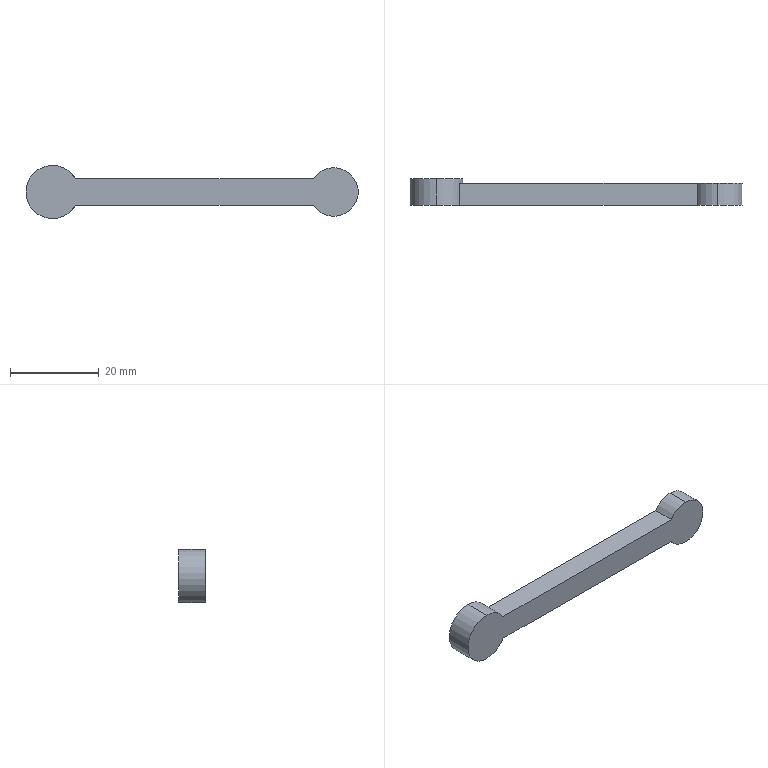Part | STEP file | 111_Default | 1 solid | 10 faces | box 75 x 6 x 12 mm | volume 2730 mm3 | cylinder 5 | plane 5 | commonest cylinder face diameters 11 x3 12 x2
STEP:
#1=CARTESIAN_POINT('',(0.,0.,0.));
#2=DIRECTION('',(0.,0.,1.));
#3=DIRECTION('',(1.,0.,0.));
#4=AXIS2_PLACEMENT_3D('',#1,#2,#3);
#5=CARTESIAN_POINT('',(31.75,0.,5.5));
#6=VERTEX_POINT('',#5);
#7=CARTESIAN_POINT('',(31.75,0.,-5.5));
#8=VERTEX_POINT('',#7);
#9=CARTESIAN_POINT('',(31.75,0.,0.));
#10=DIRECTION('',(0.,1.,0.));
#11=DIRECTION('',(0.,0.,1.));
#12=AXIS2_PLACEMENT_3D('',#9,#10,#11);
#13=CIRCLE('',#12,5.5);
#14=CARTESIAN_POINT('',(31.75,-5.,0.));
#15=DIRECTION('',(0.,1.,0.));
#16=DIRECTION('',(0.,0.,1.));
#17=AXIS2_PLACEMENT_3D('',#14,#15,#16);
#18=CYLINDRICAL_SURFACE('',#17,5.5);
#19=CARTESIAN_POINT('',(0.,5.));
#20=DIRECTION('',(1.,0.));
#21=VECTOR('',#20,1.);
#22=LINE('',#19,#21);
#23=(GEOMETRIC_REPRESENTATION_CONTEXT(2)PARAMETRIC_REPRESENTATION_CONTEXT()REPRESENTATION_CONTEXT('',''));
#24=DEFINITIONAL_REPRESENTATION('',(#22),#23);
#25=PCURVE('',#18,#24);
#26=CARTESIAN_POINT('',(31.75,0.,0.));
#27=DIRECTION('',(0.,1.,0.));
#28=DIRECTION('',(0.,0.,1.));
#29=AXIS2_PLACEMENT_3D('',#26,#27,#28);
#30=PLANE('',#29);
#31=CARTESIAN_POINT('',(0.,0.));
#32=DIRECTION('',(1.,0.));
#33=AXIS2_PLACEMENT_2D('',#31,#32);
#34=CIRCLE('',#33,5.5);
#35=(GEOMETRIC_REPRESENTATION_CONTEXT(2)PARAMETRIC_REPRESENTATION_CONTEXT()REPRESENTATION_CONTEXT('',''));
#36=DEFINITIONAL_REPRESENTATION('',(#34),#35);
#37=PCURVE('',#30,#36);
#38=SURFACE_CURVE('',#13,(#25,#37),.PCURVE_S1.);
#39=EDGE_CURVE('',#6,#8,#38,.T.);
#40=ORIENTED_EDGE('',*,*,#39,.T.);
#41=CARTESIAN_POINT('',(31.75,5.,-5.5));
#42=VERTEX_POINT('',#41);
#43=CARTESIAN_POINT('',(31.75,-5.,-5.5));
#44=DIRECTION('',(0.,1.,0.));
#45=VECTOR('',#44,1.);
#46=LINE('',#43,#45);
#47=CARTESIAN_POINT('',(3.142,0.));
#48=DIRECTION('',(0.,1.));
#49=VECTOR('',#48,1.);
#50=LINE('',#47,#49);
#51=(GEOMETRIC_REPRESENTATION_CONTEXT(2)PARAMETRIC_REPRESENTATION_CONTEXT()REPRESENTATION_CONTEXT('',''));
#52=DEFINITIONAL_REPRESENTATION('',(#50),#51);
#53=PCURVE('',#18,#52);
#54=CARTESIAN_POINT('',(31.75,-5.,0.));
#55=DIRECTION('',(0.,1.,0.));
#56=DIRECTION('',(0.,0.,1.));
#57=AXIS2_PLACEMENT_3D('',#54,#55,#56);
#58=CYLINDRICAL_SURFACE('',#57,5.5);
#59=CARTESIAN_POINT('',(3.142,0.));
#60=DIRECTION('',(0.,1.));
#61=VECTOR('',#60,1.);
#62=LINE('',#59,#61);
#63=(GEOMETRIC_REPRESENTATION_CONTEXT(2)PARAMETRIC_REPRESENTATION_CONTEXT()REPRESENTATION_CONTEXT('',''));
#64=DEFINITIONAL_REPRESENTATION('',(#62),#63);
#65=PCURVE('',#58,#64);
#66=SURFACE_CURVE('',#46,(#53,#65),.PCURVE_S1.);
#67=EDGE_CURVE('',#8,#42,#66,.T.);
#68=ORIENTED_EDGE('',*,*,#67,.T.);
#69=CARTESIAN_POINT('',(31.75,5.,5.5));
#70=VERTEX_POINT('',#69);
#71=CARTESIAN_POINT('',(31.75,5.,0.));
#72=DIRECTION('',(0.,1.,0.));
#73=DIRECTION('',(0.,0.,1.));
#74=AXIS2_PLACEMENT_3D('',#71,#72,#73);
#75=CIRCLE('',#74,5.5);
#76=CARTESIAN_POINT('',(0.,10.));
#77=DIRECTION('',(1.,0.));
#78=VECTOR('',#77,1.);
#79=LINE('',#76,#78);
#80=(GEOMETRIC_REPRESENTATION_CONTEXT(2)PARAMETRIC_REPRESENTATION_CONTEXT()REPRESENTATION_CONTEXT('',''));
#81=DEFINITIONAL_REPRESENTATION('',(#79),#80);
#82=PCURVE('',#18,#81);
#83=CARTESIAN_POINT('',(31.75,5.,0.));
#84=DIRECTION('',(0.,1.,0.));
#85=DIRECTION('',(0.,0.,1.));
#86=AXIS2_PLACEMENT_3D('',#83,#84,#85);
#87=PLANE('',#86);
#88=CARTESIAN_POINT('',(0.,0.));
#89=DIRECTION('',(1.,0.));
#90=AXIS2_PLACEMENT_2D('',#88,#89);
#91=CIRCLE('',#90,5.5);
#92=(GEOMETRIC_REPRESENTATION_CONTEXT(2)PARAMETRIC_REPRESENTATION_CONTEXT()REPRESENTATION_CONTEXT('',''));
#93=DEFINITIONAL_REPRESENTATION('',(#91),#92);
#94=PCURVE('',#87,#93);
#95=SURFACE_CURVE('',#75,(#82,#94),.PCURVE_S1.);
#96=EDGE_CURVE('',#70,#42,#95,.T.);
#97=ORIENTED_EDGE('',*,*,#96,.F.);
#98=CARTESIAN_POINT('',(31.75,-5.,5.5));
#99=DIRECTION('',(0.,1.,0.));
#100=VECTOR('',#99,1.);
#101=LINE('',#98,#100);
#102=CARTESIAN_POINT('',(0.,0.));
#103=DIRECTION('',(0.,1.));
#104=VECTOR('',#103,1.);
#105=LINE('',#102,#104);
#106=(GEOMETRIC_REPRESENTATION_CONTEXT(2)PARAMETRIC_REPRESENTATION_CONTEXT()REPRESENTATION_CONTEXT('',''));
#107=DEFINITIONAL_REPRESENTATION('',(#105),#106);
#108=PCURVE('',#18,#107);
#109=CARTESIAN_POINT('',(31.75,-5.,0.));
#110=DIRECTION('',(0.,1.,0.));
#111=DIRECTION('',(0.,0.,1.));
#112=AXIS2_PLACEMENT_3D('',#109,#110,#111);
#113=CYLINDRICAL_SURFACE('',#112,5.5);
#114=CARTESIAN_POINT('',(6.283,0.));
#115=DIRECTION('',(0.,1.));
#116=VECTOR('',#115,1.);
#117=LINE('',#114,#116);
#118=(GEOMETRIC_REPRESENTATION_CONTEXT(2)PARAMETRIC_REPRESENTATION_CONTEXT()REPRESENTATION_CONTEXT('',''));
#119=DEFINITIONAL_REPRESENTATION('',(#117),#118);
#120=PCURVE('',#113,#119);
#121=SURFACE_CURVE('',#101,(#108,#120),.PCURVE_S1.);
#122=EDGE_CURVE('',#6,#70,#121,.T.);
#123=ORIENTED_EDGE('',*,*,#122,.F.);
#124=EDGE_LOOP('',(#40,#68,#97,#123));
#125=FACE_BOUND('',#124,.T.);
#126=ADVANCED_FACE('',(#125),#18,.T.);
#127=CARTESIAN_POINT('',(27.14,0.,3.));
#128=VERTEX_POINT('',#127);
#129=CARTESIAN_POINT('',(31.75,0.,0.));
#130=DIRECTION('',(0.,1.,0.));
#131=DIRECTION('',(0.,0.,1.));
#132=AXIS2_PLACEMENT_3D('',#129,#130,#131);
#133=CIRCLE('',#132,5.5);
#134=CARTESIAN_POINT('',(0.,5.));
#135=DIRECTION('',(1.,0.));
#136=VECTOR('',#135,1.);
#137=LINE('',#134,#136);
#138=(GEOMETRIC_REPRESENTATION_CONTEXT(2)PARAMETRIC_REPRESENTATION_CONTEXT()REPRESENTATION_CONTEXT('',''));
#139=DEFINITIONAL_REPRESENTATION('',(#137),#138);
#140=PCURVE('',#113,#139);
#141=CARTESIAN_POINT('',(0.,0.));
#142=DIRECTION('',(1.,0.));
#143=AXIS2_PLACEMENT_2D('',#141,#142);
#144=CIRCLE('',#143,5.5);
#145=(GEOMETRIC_REPRESENTATION_CONTEXT(2)PARAMETRIC_REPRESENTATION_CONTEXT()REPRESENTATION_CONTEXT('',''));
#146=DEFINITIONAL_REPRESENTATION('',(#144),#145);
#147=PCURVE('',#30,#146);
#148=SURFACE_CURVE('',#133,(#140,#147),.PCURVE_S1.);
#149=EDGE_CURVE('',#128,#6,#148,.T.);
#150=ORIENTED_EDGE('',*,*,#149,.T.);
#151=ORIENTED_EDGE('',*,*,#122,.T.);
#152=CARTESIAN_POINT('',(27.14,5.,3.));
#153=VERTEX_POINT('',#152);
#154=CARTESIAN_POINT('',(31.75,5.,0.));
#155=DIRECTION('',(0.,1.,0.));
#156=DIRECTION('',(0.,0.,1.));
#157=AXIS2_PLACEMENT_3D('',#154,#155,#156);
#158=CIRCLE('',#157,5.5);
#159=CARTESIAN_POINT('',(0.,10.));
#160=DIRECTION('',(1.,0.));
#161=VECTOR('',#160,1.);
#162=LINE('',#159,#161);
#163=(GEOMETRIC_REPRESENTATION_CONTEXT(2)PARAMETRIC_REPRESENTATION_CONTEXT()REPRESENTATION_CONTEXT('',''));
#164=DEFINITIONAL_REPRESENTATION('',(#162),#163);
#165=PCURVE('',#113,#164);
#166=CARTESIAN_POINT('',(0.,0.));
#167=DIRECTION('',(1.,0.));
#168=AXIS2_PLACEMENT_2D('',#166,#167);
#169=CIRCLE('',#168,5.5);
#170=(GEOMETRIC_REPRESENTATION_CONTEXT(2)PARAMETRIC_REPRESENTATION_CONTEXT()REPRESENTATION_CONTEXT('',''));
#171=DEFINITIONAL_REPRESENTATION('',(#169),#170);
#172=PCURVE('',#87,#171);
#173=SURFACE_CURVE('',#158,(#165,#172),.PCURVE_S1.);
#174=EDGE_CURVE('',#153,#70,#173,.T.);
#175=ORIENTED_EDGE('',*,*,#174,.F.);
#176=CARTESIAN_POINT('',(27.14,-5.,3.));
#177=DIRECTION('',(0.,1.,0.));
#178=VECTOR('',#177,1.);
#179=LINE('',#176,#178);
#180=CARTESIAN_POINT('',(5.289,0.));
#181=DIRECTION('',(0.,1.));
#182=VECTOR('',#181,1.);
#183=LINE('',#180,#182);
#184=(GEOMETRIC_REPRESENTATION_CONTEXT(2)PARAMETRIC_REPRESENTATION_CONTEXT()REPRESENTATION_CONTEXT('',''));
#185=DEFINITIONAL_REPRESENTATION('',(#183),#184);
#186=PCURVE('',#113,#185);
#187=CARTESIAN_POINT('',(-26.554,-5.,3.));
#188=DIRECTION('',(0.,0.,1.));
#189=DIRECTION('',(1.,0.,0.));
#190=AXIS2_PLACEMENT_3D('',#187,#188,#189);
#191=PLANE('',#190);
#192=CARTESIAN_POINT('',(53.694,0.));
#193=DIRECTION('',(0.,1.));
#194=VECTOR('',#193,1.);
#195=LINE('',#192,#194);
#196=(GEOMETRIC_REPRESENTATION_CONTEXT(2)PARAMETRIC_REPRESENTATION_CONTEXT()REPRESENTATION_CONTEXT('',''));
#197=DEFINITIONAL_REPRESENTATION('',(#195),#196);
#198=PCURVE('',#191,#197);
#199=SURFACE_CURVE('',#179,(#186,#198),.PCURVE_S1.);
#200=EDGE_CURVE('',#128,#153,#199,.T.);
#201=ORIENTED_EDGE('',*,*,#200,.F.);
#202=EDGE_LOOP('',(#150,#151,#175,#201));
#203=FACE_BOUND('',#202,.T.);
#204=ADVANCED_FACE('',(#203),#113,.T.);
#205=CARTESIAN_POINT('',(-31.75,6.,6.));
#206=VERTEX_POINT('',#205);
#207=CARTESIAN_POINT('',(-31.75,6.,-6.));
#208=VERTEX_POINT('',#207);
#209=CARTESIAN_POINT('',(-31.75,6.,0.));
#210=DIRECTION('',(0.,1.,0.));
#211=DIRECTION('',(0.,0.,1.));
#212=AXIS2_PLACEMENT_3D('',#209,#210,#211);
#213=CIRCLE('',#212,6.);
#214=CARTESIAN_POINT('',(-31.75,5.,0.));
#215=DIRECTION('',(0.,-1.,0.));
#216=DIRECTION('',(0.,0.,-1.));
#217=AXIS2_PLACEMENT_3D('',#214,#215,#216);
#218=CYLINDRICAL_SURFACE('',#217,6.);
#219=CARTESIAN_POINT('',(3.142,-1.));
#220=DIRECTION('',(-1.,0.));
#221=VECTOR('',#220,1.);
#222=LINE('',#219,#221);
#223=(GEOMETRIC_REPRESENTATION_CONTEXT(2)PARAMETRIC_REPRESENTATION_CONTEXT()REPRESENTATION_CONTEXT('',''));
#224=DEFINITIONAL_REPRESENTATION('',(#222),#223);
#225=PCURVE('',#218,#224);
#226=CARTESIAN_POINT('',(-31.75,6.,0.));
#227=DIRECTION('',(0.,1.,0.));
#228=DIRECTION('',(0.,0.,1.));
#229=AXIS2_PLACEMENT_3D('',#226,#227,#228);
#230=PLANE('',#229);
#231=CARTESIAN_POINT('',(0.,0.));
#232=DIRECTION('',(1.,0.));
#233=AXIS2_PLACEMENT_2D('',#231,#232);
#234=CIRCLE('',#233,6.);
#235=(GEOMETRIC_REPRESENTATION_CONTEXT(2)PARAMETRIC_REPRESENTATION_CONTEXT()REPRESENTATION_CONTEXT('',''));
#236=DEFINITIONAL_REPRESENTATION('',(#234),#235);
#237=PCURVE('',#230,#236);
#238=SURFACE_CURVE('',#213,(#225,#237),.PCURVE_S1.);
#239=EDGE_CURVE('',#206,#208,#238,.T.);
#240=ORIENTED_EDGE('',*,*,#239,.F.);
#241=CARTESIAN_POINT('',(-31.75,0.,6.));
#242=VERTEX_POINT('',#241);
#243=CARTESIAN_POINT('',(-31.75,5.,6.));
#244=DIRECTION('',(0.,-1.,0.));
#245=VECTOR('',#244,1.);
#246=LINE('',#243,#245);
#247=CARTESIAN_POINT('',(3.142,0.));
#248=DIRECTION('',(0.,1.));
#249=VECTOR('',#248,1.);
#250=LINE('',#247,#249);
#251=(GEOMETRIC_REPRESENTATION_CONTEXT(2)PARAMETRIC_REPRESENTATION_CONTEXT()REPRESENTATION_CONTEXT('',''));
#252=DEFINITIONAL_REPRESENTATION('',(#250),#251);
#253=PCURVE('',#218,#252);
#254=CARTESIAN_POINT('',(-31.75,5.,0.));
#255=DIRECTION('',(0.,-1.,0.));
#256=DIRECTION('',(0.,0.,-1.));
#257=AXIS2_PLACEMENT_3D('',#254,#255,#256);
#258=CYLINDRICAL_SURFACE('',#257,6.);
#259=CARTESIAN_POINT('',(3.142,0.));
#260=DIRECTION('',(0.,1.));
#261=VECTOR('',#260,1.);
#262=LINE('',#259,#261);
#263=(GEOMETRIC_REPRESENTATION_CONTEXT(2)PARAMETRIC_REPRESENTATION_CONTEXT()REPRESENTATION_CONTEXT('',''));
#264=DEFINITIONAL_REPRESENTATION('',(#262),#263);
#265=PCURVE('',#258,#264);
#266=SURFACE_CURVE('',#246,(#253,#265),.PCURVE_S1.);
#267=EDGE_CURVE('',#206,#242,#266,.T.);
#268=ORIENTED_EDGE('',*,*,#267,.T.);
#269=CARTESIAN_POINT('',(-26.554,0.,3.));
#270=VERTEX_POINT('',#269);
#271=CARTESIAN_POINT('',(-31.75,0.,0.));
#272=DIRECTION('',(0.,1.,0.));
#273=DIRECTION('',(0.,0.,1.));
#274=AXIS2_PLACEMENT_3D('',#271,#272,#273);
#275=CIRCLE('',#274,6.);
#276=CARTESIAN_POINT('',(3.142,5.));
#277=DIRECTION('',(-1.,0.));
#278=VECTOR('',#277,1.);
#279=LINE('',#276,#278);
#280=(GEOMETRIC_REPRESENTATION_CONTEXT(2)PARAMETRIC_REPRESENTATION_CONTEXT()REPRESENTATION_CONTEXT('',''));
#281=DEFINITIONAL_REPRESENTATION('',(#279),#280);
#282=PCURVE('',#218,#281);
#283=CARTESIAN_POINT('',(0.,-63.5));
#284=DIRECTION('',(1.,0.));
#285=AXIS2_PLACEMENT_2D('',#283,#284);
#286=CIRCLE('',#285,6.);
#287=(GEOMETRIC_REPRESENTATION_CONTEXT(2)PARAMETRIC_REPRESENTATION_CONTEXT()REPRESENTATION_CONTEXT('',''));
#288=DEFINITIONAL_REPRESENTATION('',(#286),#287);
#289=PCURVE('',#30,#288);
#290=SURFACE_CURVE('',#275,(#282,#289),.PCURVE_S1.);
#291=EDGE_CURVE('',#242,#270,#290,.T.);
#292=ORIENTED_EDGE('',*,*,#291,.T.);
#293=CARTESIAN_POINT('',(-26.554,5.,3.));
#294=VERTEX_POINT('',#293);
#295=CARTESIAN_POINT('',(-26.554,-5.,3.));
#296=DIRECTION('',(0.,1.,0.));
#297=VECTOR('',#296,1.);
#298=LINE('',#295,#297);
#299=CARTESIAN_POINT('',(2.094,10.));
#300=DIRECTION('',(0.,-1.));
#301=VECTOR('',#300,1.);
#302=LINE('',#299,#301);
#303=(GEOMETRIC_REPRESENTATION_CONTEXT(2)PARAMETRIC_REPRESENTATION_CONTEXT()REPRESENTATION_CONTEXT('',''));
#304=DEFINITIONAL_REPRESENTATION('',(#302),#303);
#305=PCURVE('',#218,#304);
#306=CARTESIAN_POINT('',(0.,0.));
#307=DIRECTION('',(0.,1.));
#308=VECTOR('',#307,1.);
#309=LINE('',#306,#308);
#310=(GEOMETRIC_REPRESENTATION_CONTEXT(2)PARAMETRIC_REPRESENTATION_CONTEXT()REPRESENTATION_CONTEXT('',''));
#311=DEFINITIONAL_REPRESENTATION('',(#309),#310);
#312=PCURVE('',#191,#311);
#313=SURFACE_CURVE('',#298,(#305,#312),.PCURVE_S1.);
#314=EDGE_CURVE('',#270,#294,#313,.T.);
#315=ORIENTED_EDGE('',*,*,#314,.T.);
#316=CARTESIAN_POINT('',(-26.554,5.,-3.));
#317=VERTEX_POINT('',#316);
#318=CARTESIAN_POINT('',(-31.75,5.,0.));
#319=DIRECTION('',(0.,1.,0.));
#320=DIRECTION('',(0.,0.,1.));
#321=AXIS2_PLACEMENT_3D('',#318,#319,#320);
#322=CIRCLE('',#321,6.);
#323=CARTESIAN_POINT('',(3.142,0.));
#324=DIRECTION('',(-1.,0.));
#325=VECTOR('',#324,1.);
#326=LINE('',#323,#325);
#327=(GEOMETRIC_REPRESENTATION_CONTEXT(2)PARAMETRIC_REPRESENTATION_CONTEXT()REPRESENTATION_CONTEXT('',''));
#328=DEFINITIONAL_REPRESENTATION('',(#326),#327);
#329=PCURVE('',#218,#328);
#330=CARTESIAN_POINT('',(0.,-63.5));
#331=DIRECTION('',(1.,0.));
#332=AXIS2_PLACEMENT_2D('',#330,#331);
#333=CIRCLE('',#332,6.);
#334=(GEOMETRIC_REPRESENTATION_CONTEXT(2)PARAMETRIC_REPRESENTATION_CONTEXT()REPRESENTATION_CONTEXT('',''));
#335=DEFINITIONAL_REPRESENTATION('',(#333),#334);
#336=PCURVE('',#87,#335);
#337=SURFACE_CURVE('',#322,(#329,#336),.PCURVE_S1.);
#338=EDGE_CURVE('',#294,#317,#337,.T.);
#339=ORIENTED_EDGE('',*,*,#338,.T.);
#340=CARTESIAN_POINT('',(-26.554,0.,-3.));
#341=VERTEX_POINT('',#340);
#342=CARTESIAN_POINT('',(-26.554,-5.,-3.));
#343=DIRECTION('',(0.,1.,0.));
#344=VECTOR('',#343,1.);
#345=LINE('',#342,#344);
#346=CARTESIAN_POINT('',(1.047,10.));
#347=DIRECTION('',(0.,-1.));
#348=VECTOR('',#347,1.);
#349=LINE('',#346,#348);
#350=(GEOMETRIC_REPRESENTATION_CONTEXT(2)PARAMETRIC_REPRESENTATION_CONTEXT()REPRESENTATION_CONTEXT('',''));
#351=DEFINITIONAL_REPRESENTATION('',(#349),#350);
#352=PCURVE('',#218,#351);
#353=CARTESIAN_POINT('',(-26.554,-5.,-3.));
#354=DIRECTION('',(0.,0.,-1.));
#355=DIRECTION('',(-1.,0.,0.));
#356=AXIS2_PLACEMENT_3D('',#353,#354,#355);
#357=PLANE('',#356);
#358=CARTESIAN_POINT('',(0.,0.));
#359=DIRECTION('',(0.,1.));
#360=VECTOR('',#359,1.);
#361=LINE('',#358,#360);
#362=(GEOMETRIC_REPRESENTATION_CONTEXT(2)PARAMETRIC_REPRESENTATION_CONTEXT()REPRESENTATION_CONTEXT('',''));
#363=DEFINITIONAL_REPRESENTATION('',(#361),#362);
#364=PCURVE('',#357,#363);
#365=SURFACE_CURVE('',#345,(#352,#364),.PCURVE_S1.);
#366=EDGE_CURVE('',#341,#317,#365,.T.);
#367=ORIENTED_EDGE('',*,*,#366,.F.);
#368=CARTESIAN_POINT('',(-31.75,0.,-6.));
#369=VERTEX_POINT('',#368);
#370=CARTESIAN_POINT('',(-31.75,0.,0.));
#371=DIRECTION('',(0.,1.,0.));
#372=DIRECTION('',(0.,0.,1.));
#373=AXIS2_PLACEMENT_3D('',#370,#371,#372);
#374=CIRCLE('',#373,6.);
#375=CARTESIAN_POINT('',(3.142,5.));
#376=DIRECTION('',(-1.,0.));
#377=VECTOR('',#376,1.);
#378=LINE('',#375,#377);
#379=(GEOMETRIC_REPRESENTATION_CONTEXT(2)PARAMETRIC_REPRESENTATION_CONTEXT()REPRESENTATION_CONTEXT('',''));
#380=DEFINITIONAL_REPRESENTATION('',(#378),#379);
#381=PCURVE('',#218,#380);
#382=CARTESIAN_POINT('',(0.,-63.5));
#383=DIRECTION('',(1.,0.));
#384=AXIS2_PLACEMENT_2D('',#382,#383);
#385=CIRCLE('',#384,6.);
#386=(GEOMETRIC_REPRESENTATION_CONTEXT(2)PARAMETRIC_REPRESENTATION_CONTEXT()REPRESENTATION_CONTEXT('',''));
#387=DEFINITIONAL_REPRESENTATION('',(#385),#386);
#388=PCURVE('',#30,#387);
#389=SURFACE_CURVE('',#374,(#381,#388),.PCURVE_S1.);
#390=EDGE_CURVE('',#341,#369,#389,.T.);
#391=ORIENTED_EDGE('',*,*,#390,.T.);
#392=CARTESIAN_POINT('',(-31.75,5.,-6.));
#393=DIRECTION('',(0.,-1.,0.));
#394=VECTOR('',#393,1.);
#395=LINE('',#392,#394);
#396=CARTESIAN_POINT('',(0.,0.));
#397=DIRECTION('',(0.,1.));
#398=VECTOR('',#397,1.);
#399=LINE('',#396,#398);
#400=(GEOMETRIC_REPRESENTATION_CONTEXT(2)PARAMETRIC_REPRESENTATION_CONTEXT()REPRESENTATION_CONTEXT('',''));
#401=DEFINITIONAL_REPRESENTATION('',(#399),#400);
#402=PCURVE('',#218,#401);
#403=CARTESIAN_POINT('',(6.283,0.));
#404=DIRECTION('',(0.,1.));
#405=VECTOR('',#404,1.);
#406=LINE('',#403,#405);
#407=(GEOMETRIC_REPRESENTATION_CONTEXT(2)PARAMETRIC_REPRESENTATION_CONTEXT()REPRESENTATION_CONTEXT('',''));
#408=DEFINITIONAL_REPRESENTATION('',(#406),#407);
#409=PCURVE('',#258,#408);
#410=SURFACE_CURVE('',#395,(#402,#409),.PCURVE_S1.);
#411=EDGE_CURVE('',#208,#369,#410,.T.);
#412=ORIENTED_EDGE('',*,*,#411,.F.);
#413=EDGE_LOOP('',(#240,#268,#292,#315,#339,#367,#391,#412));
#414=FACE_BOUND('',#413,.T.);
#415=ADVANCED_FACE('',(#414),#218,.T.);
#416=ORIENTED_EDGE('',*,*,#338,.F.);
#417=CARTESIAN_POINT('',(-26.554,5.,3.));
#418=DIRECTION('',(1.,0.,0.));
#419=VECTOR('',#418,1.);
#420=LINE('',#417,#419);
#421=CARTESIAN_POINT('',(3.,-58.304));
#422=DIRECTION('',(0.,1.));
#423=VECTOR('',#422,1.);
#424=LINE('',#421,#423);
#425=(GEOMETRIC_REPRESENTATION_CONTEXT(2)PARAMETRIC_REPRESENTATION_CONTEXT()REPRESENTATION_CONTEXT('',''));
#426=DEFINITIONAL_REPRESENTATION('',(#424),#425);
#427=PCURVE('',#87,#426);
#428=CARTESIAN_POINT('',(0.,10.));
#429=DIRECTION('',(1.,0.));
#430=VECTOR('',#429,1.);
#431=LINE('',#428,#430);
#432=(GEOMETRIC_REPRESENTATION_CONTEXT(2)PARAMETRIC_REPRESENTATION_CONTEXT()REPRESENTATION_CONTEXT('',''));
#433=DEFINITIONAL_REPRESENTATION('',(#431),#432);
#434=PCURVE('',#191,#433);
#435=SURFACE_CURVE('',#420,(#427,#434),.PCURVE_S1.);
#436=EDGE_CURVE('',#294,#153,#435,.T.);
#437=ORIENTED_EDGE('',*,*,#436,.T.);
#438=ORIENTED_EDGE('',*,*,#174,.T.);
#439=ORIENTED_EDGE('',*,*,#96,.T.);
#440=CARTESIAN_POINT('',(27.14,5.,-3.));
#441=VERTEX_POINT('',#440);
#442=CARTESIAN_POINT('',(31.75,5.,0.));
#443=DIRECTION('',(0.,1.,0.));
#444=DIRECTION('',(0.,0.,1.));
#445=AXIS2_PLACEMENT_3D('',#442,#443,#444);
#446=CIRCLE('',#445,5.5);
#447=CARTESIAN_POINT('',(0.,0.));
#448=DIRECTION('',(1.,0.));
#449=AXIS2_PLACEMENT_2D('',#447,#448);
#450=CIRCLE('',#449,5.5);
#451=(GEOMETRIC_REPRESENTATION_CONTEXT(2)PARAMETRIC_REPRESENTATION_CONTEXT()REPRESENTATION_CONTEXT('',''));
#452=DEFINITIONAL_REPRESENTATION('',(#450),#451);
#453=PCURVE('',#87,#452);
#454=CARTESIAN_POINT('',(0.,10.));
#455=DIRECTION('',(1.,0.));
#456=VECTOR('',#455,1.);
#457=LINE('',#454,#456);
#458=(GEOMETRIC_REPRESENTATION_CONTEXT(2)PARAMETRIC_REPRESENTATION_CONTEXT()REPRESENTATION_CONTEXT('',''));
#459=DEFINITIONAL_REPRESENTATION('',(#457),#458);
#460=PCURVE('',#58,#459);
#461=SURFACE_CURVE('',#446,(#453,#460),.PCURVE_S1.);
#462=EDGE_CURVE('',#42,#441,#461,.T.);
#463=ORIENTED_EDGE('',*,*,#462,.T.);
#464=CARTESIAN_POINT('',(-26.554,5.,-3.));
#465=DIRECTION('',(-1.,0.,0.));
#466=VECTOR('',#465,1.);
#467=LINE('',#464,#466);
#468=CARTESIAN_POINT('',(-3.,-58.304));
#469=DIRECTION('',(0.,-1.));
#470=VECTOR('',#469,1.);
#471=LINE('',#468,#470);
#472=(GEOMETRIC_REPRESENTATION_CONTEXT(2)PARAMETRIC_REPRESENTATION_CONTEXT()REPRESENTATION_CONTEXT('',''));
#473=DEFINITIONAL_REPRESENTATION('',(#471),#472);
#474=PCURVE('',#87,#473);
#475=CARTESIAN_POINT('',(0.,10.));
#476=DIRECTION('',(1.,0.));
#477=VECTOR('',#476,1.);
#478=LINE('',#475,#477);
#479=(GEOMETRIC_REPRESENTATION_CONTEXT(2)PARAMETRIC_REPRESENTATION_CONTEXT()REPRESENTATION_CONTEXT('',''));
#480=DEFINITIONAL_REPRESENTATION('',(#478),#479);
#481=PCURVE('',#357,#480);
#482=SURFACE_CURVE('',#467,(#474,#481),.PCURVE_S1.);
#483=EDGE_CURVE('',#441,#317,#482,.T.);
#484=ORIENTED_EDGE('',*,*,#483,.T.);
#485=EDGE_LOOP('',(#416,#437,#438,#439,#463,#484));
#486=FACE_BOUND('',#485,.T.);
#487=ADVANCED_FACE('',(#486),#87,.T.);
#488=ORIENTED_EDGE('',*,*,#390,.F.);
#489=CARTESIAN_POINT('',(27.14,0.,-3.));
#490=VERTEX_POINT('',#489);
#491=CARTESIAN_POINT('',(31.75,0.,-3.));
#492=DIRECTION('',(-1.,0.,0.));
#493=VECTOR('',#492,1.);
#494=LINE('',#491,#493);
#495=CARTESIAN_POINT('',(-3.,0.));
#496=DIRECTION('',(0.,-1.));
#497=VECTOR('',#496,1.);
#498=LINE('',#495,#497);
#499=(GEOMETRIC_REPRESENTATION_CONTEXT(2)PARAMETRIC_REPRESENTATION_CONTEXT()REPRESENTATION_CONTEXT('',''));
#500=DEFINITIONAL_REPRESENTATION('',(#498),#499);
#501=PCURVE('',#30,#500);
#502=CARTESIAN_POINT('',(-58.304,5.));
#503=DIRECTION('',(1.,0.));
#504=VECTOR('',#503,1.);
#505=LINE('',#502,#504);
#506=(GEOMETRIC_REPRESENTATION_CONTEXT(2)PARAMETRIC_REPRESENTATION_CONTEXT()REPRESENTATION_CONTEXT('',''));
#507=DEFINITIONAL_REPRESENTATION('',(#505),#506);
#508=PCURVE('',#357,#507);
#509=SURFACE_CURVE('',#494,(#501,#508),.PCURVE_S1.);
#510=EDGE_CURVE('',#490,#341,#509,.T.);
#511=ORIENTED_EDGE('',*,*,#510,.F.);
#512=CARTESIAN_POINT('',(31.75,0.,0.));
#513=DIRECTION('',(0.,1.,0.));
#514=DIRECTION('',(0.,0.,1.));
#515=AXIS2_PLACEMENT_3D('',#512,#513,#514);
#516=CIRCLE('',#515,5.5);
#517=CARTESIAN_POINT('',(0.,0.));
#518=DIRECTION('',(1.,0.));
#519=AXIS2_PLACEMENT_2D('',#517,#518);
#520=CIRCLE('',#519,5.5);
#521=(GEOMETRIC_REPRESENTATION_CONTEXT(2)PARAMETRIC_REPRESENTATION_CONTEXT()REPRESENTATION_CONTEXT('',''));
#522=DEFINITIONAL_REPRESENTATION('',(#520),#521);
#523=PCURVE('',#30,#522);
#524=CARTESIAN_POINT('',(0.,5.));
#525=DIRECTION('',(1.,0.));
#526=VECTOR('',#525,1.);
#527=LINE('',#524,#526);
#528=(GEOMETRIC_REPRESENTATION_CONTEXT(2)PARAMETRIC_REPRESENTATION_CONTEXT()REPRESENTATION_CONTEXT('',''));
#529=DEFINITIONAL_REPRESENTATION('',(#527),#528);
#530=PCURVE('',#58,#529);
#531=SURFACE_CURVE('',#516,(#523,#530),.PCURVE_S1.);
#532=EDGE_CURVE('',#8,#490,#531,.T.);
#533=ORIENTED_EDGE('',*,*,#532,.F.);
#534=ORIENTED_EDGE('',*,*,#39,.F.);
#535=ORIENTED_EDGE('',*,*,#149,.F.);
#536=CARTESIAN_POINT('',(31.75,0.,3.));
#537=DIRECTION('',(1.,0.,0.));
#538=VECTOR('',#537,1.);
#539=LINE('',#536,#538);
#540=CARTESIAN_POINT('',(3.,0.));
#541=DIRECTION('',(0.,1.));
#542=VECTOR('',#541,1.);
#543=LINE('',#540,#542);
#544=(GEOMETRIC_REPRESENTATION_CONTEXT(2)PARAMETRIC_REPRESENTATION_CONTEXT()REPRESENTATION_CONTEXT('',''));
#545=DEFINITIONAL_REPRESENTATION('',(#543),#544);
#546=PCURVE('',#30,#545);
#547=CARTESIAN_POINT('',(58.304,5.));
#548=DIRECTION('',(1.,0.));
#549=VECTOR('',#548,1.);
#550=LINE('',#547,#549);
#551=(GEOMETRIC_REPRESENTATION_CONTEXT(2)PARAMETRIC_REPRESENTATION_CONTEXT()REPRESENTATION_CONTEXT('',''));
#552=DEFINITIONAL_REPRESENTATION('',(#550),#551);
#553=PCURVE('',#191,#552);
#554=SURFACE_CURVE('',#539,(#546,#553),.PCURVE_S1.);
#555=EDGE_CURVE('',#270,#128,#554,.T.);
#556=ORIENTED_EDGE('',*,*,#555,.F.);
#557=ORIENTED_EDGE('',*,*,#291,.F.);
#558=CARTESIAN_POINT('',(-31.75,0.,0.));
#559=DIRECTION('',(0.,1.,0.));
#560=DIRECTION('',(0.,0.,1.));
#561=AXIS2_PLACEMENT_3D('',#558,#559,#560);
#562=CIRCLE('',#561,6.);
#563=CARTESIAN_POINT('',(0.,-63.5));
#564=DIRECTION('',(1.,0.));
#565=AXIS2_PLACEMENT_2D('',#563,#564);
#566=CIRCLE('',#565,6.);
#567=(GEOMETRIC_REPRESENTATION_CONTEXT(2)PARAMETRIC_REPRESENTATION_CONTEXT()REPRESENTATION_CONTEXT('',''));
#568=DEFINITIONAL_REPRESENTATION('',(#566),#567);
#569=PCURVE('',#30,#568);
#570=CARTESIAN_POINT('',(9.425,5.));
#571=DIRECTION('',(-1.,0.));
#572=VECTOR('',#571,1.);
#573=LINE('',#570,#572);
#574=(GEOMETRIC_REPRESENTATION_CONTEXT(2)PARAMETRIC_REPRESENTATION_CONTEXT()REPRESENTATION_CONTEXT('',''));
#575=DEFINITIONAL_REPRESENTATION('',(#573),#574);
#576=PCURVE('',#258,#575);
#577=SURFACE_CURVE('',#562,(#569,#576),.PCURVE_S1.);
#578=EDGE_CURVE('',#369,#242,#577,.T.);
#579=ORIENTED_EDGE('',*,*,#578,.F.);
#580=EDGE_LOOP('',(#488,#511,#533,#534,#535,#556,#557,#579));
#581=FACE_BOUND('',#580,.T.);
#582=ADVANCED_FACE('',(#581),#30,.F.);
#583=ORIENTED_EDGE('',*,*,#267,.F.);
#584=CARTESIAN_POINT('',(-31.75,6.,0.));
#585=DIRECTION('',(0.,1.,0.));
#586=DIRECTION('',(0.,0.,1.));
#587=AXIS2_PLACEMENT_3D('',#584,#585,#586);
#588=CIRCLE('',#587,6.);
#589=CARTESIAN_POINT('',(9.425,-1.));
#590=DIRECTION('',(-1.,0.));
#591=VECTOR('',#590,1.);
#592=LINE('',#589,#591);
#593=(GEOMETRIC_REPRESENTATION_CONTEXT(2)PARAMETRIC_REPRESENTATION_CONTEXT()REPRESENTATION_CONTEXT('',''));
#594=DEFINITIONAL_REPRESENTATION('',(#592),#593);
#595=PCURVE('',#258,#594);
#596=CARTESIAN_POINT('',(0.,0.));
#597=DIRECTION('',(1.,0.));
#598=AXIS2_PLACEMENT_2D('',#596,#597);
#599=CIRCLE('',#598,6.);
#600=(GEOMETRIC_REPRESENTATION_CONTEXT(2)PARAMETRIC_REPRESENTATION_CONTEXT()REPRESENTATION_CONTEXT('',''));
#601=DEFINITIONAL_REPRESENTATION('',(#599),#600);
#602=PCURVE('',#230,#601);
#603=SURFACE_CURVE('',#588,(#595,#602),.PCURVE_S1.);
#604=EDGE_CURVE('',#208,#206,#603,.T.);
#605=ORIENTED_EDGE('',*,*,#604,.F.);
#606=ORIENTED_EDGE('',*,*,#411,.T.);
#607=ORIENTED_EDGE('',*,*,#578,.T.);
#608=EDGE_LOOP('',(#583,#605,#606,#607));
#609=FACE_BOUND('',#608,.T.);
#610=ADVANCED_FACE('',(#609),#258,.T.);
#611=ORIENTED_EDGE('',*,*,#510,.T.);
#612=ORIENTED_EDGE('',*,*,#366,.T.);
#613=ORIENTED_EDGE('',*,*,#483,.F.);
#614=CARTESIAN_POINT('',(27.14,-5.,-3.));
#615=DIRECTION('',(0.,1.,0.));
#616=VECTOR('',#615,1.);
#617=LINE('',#614,#616);
#618=CARTESIAN_POINT('',(-53.694,0.));
#619=DIRECTION('',(0.,1.));
#620=VECTOR('',#619,1.);
#621=LINE('',#618,#620);
#622=(GEOMETRIC_REPRESENTATION_CONTEXT(2)PARAMETRIC_REPRESENTATION_CONTEXT()REPRESENTATION_CONTEXT('',''));
#623=DEFINITIONAL_REPRESENTATION('',(#621),#622);
#624=PCURVE('',#357,#623);
#625=CARTESIAN_POINT('',(4.135,0.));
#626=DIRECTION('',(0.,1.));
#627=VECTOR('',#626,1.);
#628=LINE('',#625,#627);
#629=(GEOMETRIC_REPRESENTATION_CONTEXT(2)PARAMETRIC_REPRESENTATION_CONTEXT()REPRESENTATION_CONTEXT('',''));
#630=DEFINITIONAL_REPRESENTATION('',(#628),#629);
#631=PCURVE('',#58,#630);
#632=SURFACE_CURVE('',#617,(#624,#631),.PCURVE_S1.);
#633=EDGE_CURVE('',#490,#441,#632,.T.);
#634=ORIENTED_EDGE('',*,*,#633,.F.);
#635=EDGE_LOOP('',(#611,#612,#613,#634));
#636=FACE_BOUND('',#635,.T.);
#637=ADVANCED_FACE('',(#636),#357,.T.);
#638=ORIENTED_EDGE('',*,*,#67,.F.);
#639=ORIENTED_EDGE('',*,*,#532,.T.);
#640=ORIENTED_EDGE('',*,*,#633,.T.);
#641=ORIENTED_EDGE('',*,*,#462,.F.);
#642=EDGE_LOOP('',(#638,#639,#640,#641));
#643=FACE_BOUND('',#642,.T.);
#644=ADVANCED_FACE('',(#643),#58,.T.);
#645=ORIENTED_EDGE('',*,*,#555,.T.);
#646=ORIENTED_EDGE('',*,*,#200,.T.);
#647=ORIENTED_EDGE('',*,*,#436,.F.);
#648=ORIENTED_EDGE('',*,*,#314,.F.);
#649=EDGE_LOOP('',(#645,#646,#647,#648));
#650=FACE_BOUND('',#649,.T.);
#651=ADVANCED_FACE('',(#650),#191,.T.);
#652=ORIENTED_EDGE('',*,*,#604,.T.);
#653=ORIENTED_EDGE('',*,*,#239,.T.);
#654=EDGE_LOOP('',(#652,#653));
#655=FACE_BOUND('',#654,.T.);
#656=ADVANCED_FACE('',(#655),#230,.T.);
#657=CLOSED_SHELL('',(#126,#204,#415,#487,#582,#610,#637,#644,#651,#656));
#658=MANIFOLD_SOLID_BREP('',#657);
#659=(LENGTH_UNIT()NAMED_UNIT(*)SI_UNIT(.MILLI.,.METRE.));
#660=UNCERTAINTY_MEASURE_WITH_UNIT(LENGTH_MEASURE(0.0000001),#659,'','');
#661=(NAMED_UNIT(*)PLANE_ANGLE_UNIT()SI_UNIT($,.RADIAN.));
#662=(NAMED_UNIT(*)SI_UNIT($,.STERADIAN.)SOLID_ANGLE_UNIT());
#663=(GEOMETRIC_REPRESENTATION_CONTEXT(3)GLOBAL_UNCERTAINTY_ASSIGNED_CONTEXT((#660))GLOBAL_UNIT_ASSIGNED_CONTEXT((#659,#661,#662))REPRESENTATION_CONTEXT('',''));
#664=ADVANCED_BREP_SHAPE_REPRESENTATION('',(#4,#658),#663);